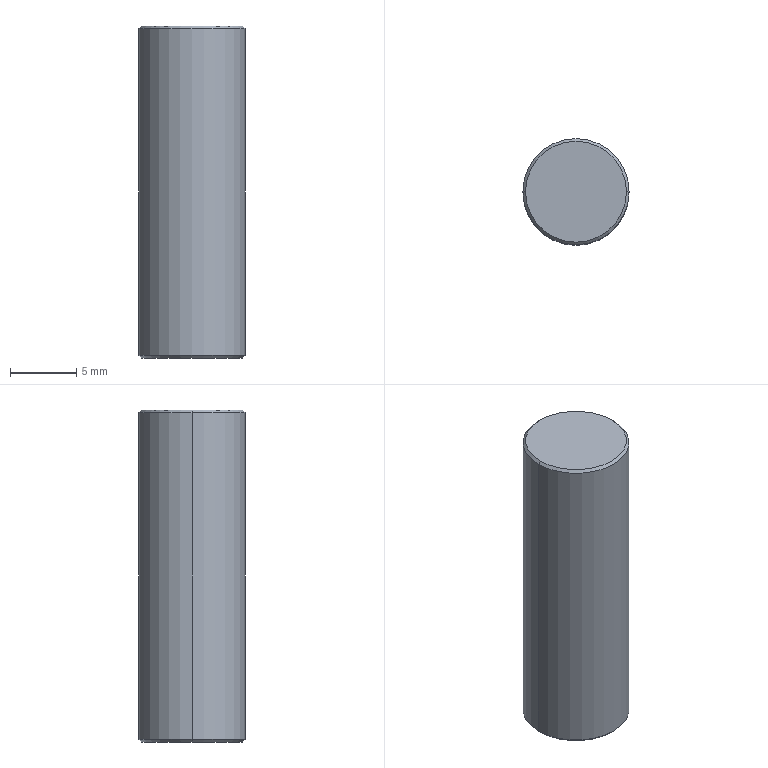Part | NX | features BREP 1 | 1 solid | 8 faces | box 8 x 8 x 25 mm | volume 1256 mm3 | cone 4 | cylinder 2 | plane 2 | commonest cylinder face diameters 8 x2
STEP:
#1=CARTESIAN_POINT('',(3.8,0.,12.5));
#2=VERTEX_POINT('',#1);
#3=CARTESIAN_POINT('',(-3.8,0.,12.5));
#4=VERTEX_POINT('',#3);
#5=CARTESIAN_POINT('',(0.,0.,12.5));
#6=DIRECTION('',(0.,0.,1.));
#7=DIRECTION('',(1.,0.,0.));
#8=AXIS2_PLACEMENT_3D('',#5,#6,#7);
#9=CIRCLE('',#8,3.8);
#10=EDGE_CURVE('',#2,#4,#9,.T.);
#11=ORIENTED_EDGE('',*,*,#10,.F.);
#12=CARTESIAN_POINT('',(4.,0.,12.3));
#13=VERTEX_POINT('',#12);
#14=CARTESIAN_POINT('',(3.8,0.,12.5));
#15=DIRECTION('',(0.7071,0.,-0.7071));
#16=VECTOR('',#15,1000.);
#17=LINE('',#14,#16);
#18=EDGE_CURVE('',#2,#13,#17,.T.);
#19=ORIENTED_EDGE('',*,*,#18,.T.);
#20=CARTESIAN_POINT('',(-4.,0.,12.3));
#21=VERTEX_POINT('',#20);
#22=CARTESIAN_POINT('',(0.,0.,12.3));
#23=DIRECTION('',(0.,0.,-1.));
#24=DIRECTION('',(1.,0.,0.));
#25=AXIS2_PLACEMENT_3D('',#22,#23,#24);
#26=CIRCLE('',#25,4.);
#27=EDGE_CURVE('',#21,#13,#26,.T.);
#28=ORIENTED_EDGE('',*,*,#27,.F.);
#29=CARTESIAN_POINT('',(-3.8,0.,12.5));
#30=DIRECTION('',(-0.7071,0.,-0.7071));
#31=VECTOR('',#30,1000.);
#32=LINE('',#29,#31);
#33=EDGE_CURVE('',#4,#21,#32,.T.);
#34=ORIENTED_EDGE('',*,*,#33,.F.);
#35=EDGE_LOOP('',(#11,#19,#28,#34));
#36=FACE_BOUND('',#35,.T.);
#37=CARTESIAN_POINT('',(0.,0.,12.5));
#38=DIRECTION('',(0.,0.,-1.));
#39=DIRECTION('',(-1.,0.,0.));
#40=AXIS2_PLACEMENT_3D('',#37,#38,#39);
#41=CONICAL_SURFACE('',#40,3.8,0.7854);
#42=ADVANCED_FACE('',(#36),#41,.T.);
#43=CARTESIAN_POINT('',(-3.8,0.,-12.5));
#44=VERTEX_POINT('',#43);
#45=CARTESIAN_POINT('',(3.8,0.,-12.5));
#46=VERTEX_POINT('',#45);
#47=CARTESIAN_POINT('',(0.,0.,-12.5));
#48=DIRECTION('',(0.,0.,-1.));
#49=DIRECTION('',(1.,0.,0.));
#50=AXIS2_PLACEMENT_3D('',#47,#48,#49);
#51=CIRCLE('',#50,3.8);
#52=EDGE_CURVE('',#44,#46,#51,.T.);
#53=ORIENTED_EDGE('',*,*,#52,.F.);
#54=CARTESIAN_POINT('',(-4.,0.,-12.3));
#55=VERTEX_POINT('',#54);
#56=CARTESIAN_POINT('',(-4.,0.,-12.3));
#57=DIRECTION('',(-0.7071,0.,0.7071));
#58=VECTOR('',#57,1000.);
#59=LINE('',#56,#58);
#60=EDGE_CURVE('',#55,#44,#59,.F.);
#61=ORIENTED_EDGE('',*,*,#60,.F.);
#62=CARTESIAN_POINT('',(4.,0.,-12.3));
#63=VERTEX_POINT('',#62);
#64=CARTESIAN_POINT('',(0.,0.,-12.3));
#65=DIRECTION('',(0.,0.,1.));
#66=DIRECTION('',(1.,0.,0.));
#67=AXIS2_PLACEMENT_3D('',#64,#65,#66);
#68=CIRCLE('',#67,4.);
#69=EDGE_CURVE('',#63,#55,#68,.T.);
#70=ORIENTED_EDGE('',*,*,#69,.F.);
#71=CARTESIAN_POINT('',(4.,0.,-12.3));
#72=DIRECTION('',(0.7071,0.,0.7071));
#73=VECTOR('',#72,1000.);
#74=LINE('',#71,#73);
#75=EDGE_CURVE('',#63,#46,#74,.F.);
#76=ORIENTED_EDGE('',*,*,#75,.T.);
#77=EDGE_LOOP('',(#53,#61,#70,#76));
#78=FACE_BOUND('',#77,.T.);
#79=CARTESIAN_POINT('',(0.,0.,-12.3));
#80=DIRECTION('',(0.,0.,1.));
#81=DIRECTION('',(1.,0.,0.));
#82=AXIS2_PLACEMENT_3D('',#79,#80,#81);
#83=CONICAL_SURFACE('',#82,4.,0.7854);
#84=ADVANCED_FACE('',(#78),#83,.T.);
#85=ORIENTED_EDGE('',*,*,#27,.T.);
#86=CARTESIAN_POINT('',(4.,0.,12.5));
#87=DIRECTION('',(0.,0.,-1.));
#88=VECTOR('',#87,1000.);
#89=LINE('',#86,#88);
#90=EDGE_CURVE('',#13,#63,#89,.T.);
#91=ORIENTED_EDGE('',*,*,#90,.T.);
#92=ORIENTED_EDGE('',*,*,#69,.T.);
#93=CARTESIAN_POINT('',(-4.,0.,12.5));
#94=DIRECTION('',(0.,0.,-1.));
#95=VECTOR('',#94,1000.);
#96=LINE('',#93,#95);
#97=EDGE_CURVE('',#21,#55,#96,.T.);
#98=ORIENTED_EDGE('',*,*,#97,.F.);
#99=EDGE_LOOP('',(#85,#91,#92,#98));
#100=FACE_BOUND('',#99,.T.);
#101=CARTESIAN_POINT('',(0.,0.,12.5));
#102=DIRECTION('',(0.,0.,-1.));
#103=DIRECTION('',(-1.,0.,0.));
#104=AXIS2_PLACEMENT_3D('',#101,#102,#103);
#105=CYLINDRICAL_SURFACE('',#104,4.);
#106=ADVANCED_FACE('',(#100),#105,.T.);
#107=ORIENTED_EDGE('',*,*,#90,.F.);
#108=CARTESIAN_POINT('',(0.,0.,12.3));
#109=DIRECTION('',(0.,0.,-1.));
#110=DIRECTION('',(1.,0.,0.));
#111=AXIS2_PLACEMENT_3D('',#108,#109,#110);
#112=CIRCLE('',#111,4.);
#113=EDGE_CURVE('',#13,#21,#112,.T.);
#114=ORIENTED_EDGE('',*,*,#113,.T.);
#115=ORIENTED_EDGE('',*,*,#97,.T.);
#116=CARTESIAN_POINT('',(0.,0.,-12.3));
#117=DIRECTION('',(0.,0.,1.));
#118=DIRECTION('',(1.,0.,0.));
#119=AXIS2_PLACEMENT_3D('',#116,#117,#118);
#120=CIRCLE('',#119,4.);
#121=EDGE_CURVE('',#55,#63,#120,.T.);
#122=ORIENTED_EDGE('',*,*,#121,.T.);
#123=EDGE_LOOP('',(#107,#114,#115,#122));
#124=FACE_BOUND('',#123,.T.);
#125=CARTESIAN_POINT('',(0.,0.,12.5));
#126=DIRECTION('',(0.,0.,-1.));
#127=DIRECTION('',(-1.,0.,0.));
#128=AXIS2_PLACEMENT_3D('',#125,#126,#127);
#129=CYLINDRICAL_SURFACE('',#128,4.);
#130=ADVANCED_FACE('',(#124),#129,.T.);
#131=CARTESIAN_POINT('',(0.,0.,12.5));
#132=DIRECTION('',(0.,0.,1.));
#133=DIRECTION('',(1.,0.,0.));
#134=AXIS2_PLACEMENT_3D('',#131,#132,#133);
#135=CIRCLE('',#134,3.8);
#136=EDGE_CURVE('',#4,#2,#135,.T.);
#137=ORIENTED_EDGE('',*,*,#136,.T.);
#138=ORIENTED_EDGE('',*,*,#10,.T.);
#139=EDGE_LOOP('',(#137,#138));
#140=FACE_BOUND('',#139,.T.);
#141=CARTESIAN_POINT('',(0.,0.,12.5));
#142=DIRECTION('',(0.,0.,1.));
#143=DIRECTION('',(1.,0.,0.));
#144=AXIS2_PLACEMENT_3D('',#141,#142,#143);
#145=PLANE('',#144);
#146=ADVANCED_FACE('',(#140),#145,.T.);
#147=CARTESIAN_POINT('',(0.,0.,-12.5));
#148=DIRECTION('',(0.,0.,-1.));
#149=DIRECTION('',(1.,0.,0.));
#150=AXIS2_PLACEMENT_3D('',#147,#148,#149);
#151=CIRCLE('',#150,3.8);
#152=EDGE_CURVE('',#46,#44,#151,.T.);
#153=ORIENTED_EDGE('',*,*,#152,.T.);
#154=ORIENTED_EDGE('',*,*,#52,.T.);
#155=EDGE_LOOP('',(#153,#154));
#156=FACE_BOUND('',#155,.T.);
#157=CARTESIAN_POINT('',(0.,0.,-12.5));
#158=DIRECTION('',(0.,0.,1.));
#159=DIRECTION('',(1.,0.,0.));
#160=AXIS2_PLACEMENT_3D('',#157,#158,#159);
#161=PLANE('',#160);
#162=ADVANCED_FACE('',(#156),#161,.F.);
#163=ORIENTED_EDGE('',*,*,#60,.T.);
#164=ORIENTED_EDGE('',*,*,#152,.F.);
#165=ORIENTED_EDGE('',*,*,#75,.F.);
#166=ORIENTED_EDGE('',*,*,#121,.F.);
#167=EDGE_LOOP('',(#163,#164,#165,#166));
#168=FACE_BOUND('',#167,.T.);
#169=CARTESIAN_POINT('',(0.,0.,-12.3));
#170=DIRECTION('',(0.,0.,1.));
#171=DIRECTION('',(1.,0.,0.));
#172=AXIS2_PLACEMENT_3D('',#169,#170,#171);
#173=CONICAL_SURFACE('',#172,4.,0.7854);
#174=ADVANCED_FACE('',(#168),#173,.T.);
#175=ORIENTED_EDGE('',*,*,#18,.F.);
#176=ORIENTED_EDGE('',*,*,#136,.F.);
#177=ORIENTED_EDGE('',*,*,#33,.T.);
#178=ORIENTED_EDGE('',*,*,#113,.F.);
#179=EDGE_LOOP('',(#175,#176,#177,#178));
#180=FACE_BOUND('',#179,.T.);
#181=CARTESIAN_POINT('',(0.,0.,12.5));
#182=DIRECTION('',(0.,0.,-1.));
#183=DIRECTION('',(-1.,0.,0.));
#184=AXIS2_PLACEMENT_3D('',#181,#182,#183);
#185=CONICAL_SURFACE('',#184,3.8,0.7854);
#186=ADVANCED_FACE('',(#180),#185,.T.);
#187=CLOSED_SHELL('',(#42,#84,#106,#130,#146,#162,#174,#186));
#188=MANIFOLD_SOLID_BREP('',#187);
#189=(LENGTH_UNIT()NAMED_UNIT(*)SI_UNIT(.MILLI.,.METRE.));
#190=UNCERTAINTY_MEASURE_WITH_UNIT(LENGTH_MEASURE(0.00001),#189,'','');
#191=(NAMED_UNIT(*)PLANE_ANGLE_UNIT()SI_UNIT($,.RADIAN.));
#192=(NAMED_UNIT(*)SI_UNIT($,.STERADIAN.)SOLID_ANGLE_UNIT());
#193=(GEOMETRIC_REPRESENTATION_CONTEXT(3)GLOBAL_UNCERTAINTY_ASSIGNED_CONTEXT((#190))GLOBAL_UNIT_ASSIGNED_CONTEXT((#189,#191,#192))REPRESENTATION_CONTEXT('',''));
#194=ADVANCED_BREP_SHAPE_REPRESENTATION('',(#188),#193);